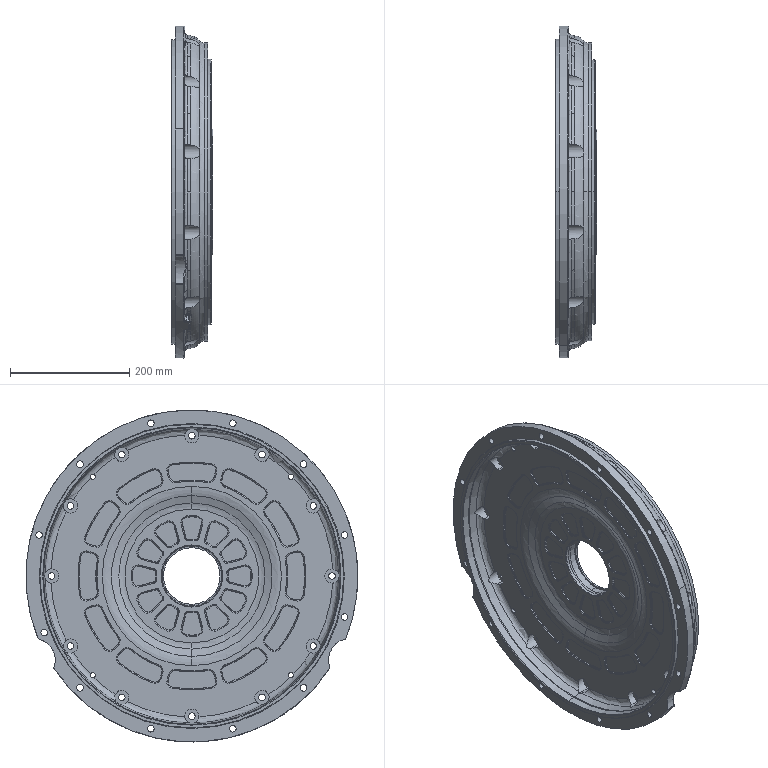Part | SolidWorks | features BaseBody 1 | 1 solid | 954 faces | box 70 x 556.6 x 556.6 mm | volume 4634291 mm3 | cylinder 369 | torus 349 | plane 164 | cone 44 | spline 18 | sphere 10 | commonest cylinder face diameters 2 x96 20 x72 11 x48 24 x38 10 x24 120 x12